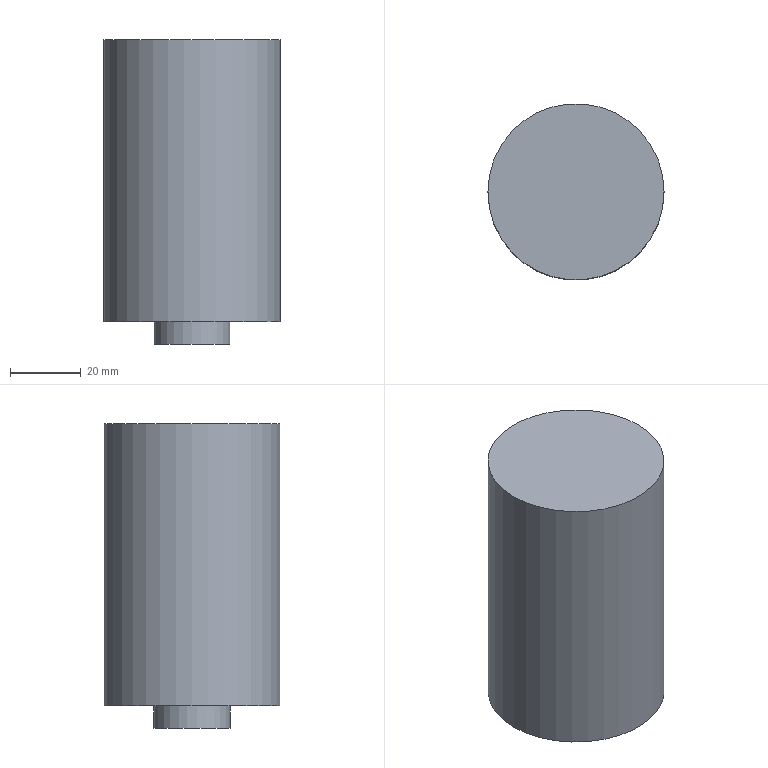Part | NX | features solid 2 | 1 solid | 5 faces | box 49.947 x 49.947 x 86.345 mm | volume 159066 mm3 | plane 3 | cylinder 2 | commonest cylinder face diameters 21.573 x1 49.947 x1
STEP:
#1=CARTESIAN_POINT('',(-1470.026,-350.026,-125.));
#2=VERTEX_POINT('',#1);
#3=CARTESIAN_POINT('',(-1495.,-350.026,-125.));
#4=DIRECTION('',(0.,0.,1.));
#5=DIRECTION('',(1.,0.,0.));
#6=AXIS2_PLACEMENT_3D('',#3,#4,#5);
#7=CIRCLE('',#6,24.974);
#8=EDGE_CURVE('',#2,#2,#7,.F.);
#9=ORIENTED_EDGE('',*,*,#8,.T.);
#10=EDGE_LOOP('',(#9));
#11=FACE_BOUND('',#10,.T.);
#12=CARTESIAN_POINT('',(-1470.026,-350.026,-205.));
#13=VERTEX_POINT('',#12);
#14=CARTESIAN_POINT('',(-1495.,-350.026,-205.));
#15=DIRECTION('',(0.,0.,1.));
#16=DIRECTION('',(1.,0.,0.));
#17=AXIS2_PLACEMENT_3D('',#14,#15,#16);
#18=CIRCLE('',#17,24.974);
#19=EDGE_CURVE('',#13,#13,#18,.F.);
#20=ORIENTED_EDGE('',*,*,#19,.F.);
#21=EDGE_LOOP('',(#20));
#22=FACE_BOUND('',#21,.T.);
#23=CARTESIAN_POINT('',(-1495.,-350.026,-141.55));
#24=DIRECTION('',(0.,0.,-1.));
#25=DIRECTION('',(0.,1.,0.));
#26=AXIS2_PLACEMENT_3D('',#23,#24,#25);
#27=CYLINDRICAL_SURFACE('',#26,24.974);
#28=ADVANCED_FACE('',(#11,#22),#27,.T.);
#29=CARTESIAN_POINT('',(-1495.,-360.813,-205.));
#30=VERTEX_POINT('',#29);
#31=CARTESIAN_POINT('',(-1495.,-350.026,-205.));
#32=DIRECTION('',(0.,0.,-1.));
#33=DIRECTION('',(0.,-1.,0.));
#34=AXIS2_PLACEMENT_3D('',#31,#32,#33);
#35=CIRCLE('',#34,10.787);
#36=EDGE_CURVE('',#30,#30,#35,.T.);
#37=ORIENTED_EDGE('',*,*,#36,.F.);
#38=EDGE_LOOP('',(#37));
#39=FACE_BOUND('',#38,.T.);
#40=ORIENTED_EDGE('',*,*,#19,.T.);
#41=EDGE_LOOP('',(#40));
#42=FACE_BOUND('',#41,.T.);
#43=CARTESIAN_POINT('',(-1495.,-350.026,-205.));
#44=DIRECTION('',(0.,0.,1.));
#45=DIRECTION('',(0.,-1.,0.));
#46=AXIS2_PLACEMENT_3D('',#43,#44,#45);
#47=PLANE('',#46);
#48=ADVANCED_FACE('',(#39,#42),#47,.F.);
#49=CARTESIAN_POINT('',(-1495.,-360.813,-211.345));
#50=VERTEX_POINT('',#49);
#51=CARTESIAN_POINT('',(-1495.,-350.026,-211.345));
#52=DIRECTION('',(0.,0.,-1.));
#53=DIRECTION('',(0.,-1.,0.));
#54=AXIS2_PLACEMENT_3D('',#51,#52,#53);
#55=CIRCLE('',#54,10.787);
#56=EDGE_CURVE('',#50,#50,#55,.T.);
#57=ORIENTED_EDGE('',*,*,#56,.F.);
#58=EDGE_LOOP('',(#57));
#59=FACE_BOUND('',#58,.T.);
#60=ORIENTED_EDGE('',*,*,#36,.T.);
#61=EDGE_LOOP('',(#60));
#62=FACE_BOUND('',#61,.T.);
#63=CARTESIAN_POINT('',(-1495.,-350.026,-211.345));
#64=DIRECTION('',(0.,0.,1.));
#65=DIRECTION('',(0.,-1.,0.));
#66=AXIS2_PLACEMENT_3D('',#63,#64,#65);
#67=CYLINDRICAL_SURFACE('',#66,10.787);
#68=ADVANCED_FACE('',(#59,#62),#67,.T.);
#69=ORIENTED_EDGE('',*,*,#56,.T.);
#70=EDGE_LOOP('',(#69));
#71=FACE_BOUND('',#70,.T.);
#72=CARTESIAN_POINT('',(-1495.,-350.026,-211.345));
#73=DIRECTION('',(0.,0.,1.));
#74=DIRECTION('',(0.,-1.,0.));
#75=AXIS2_PLACEMENT_3D('',#72,#73,#74);
#76=PLANE('',#75);
#77=ADVANCED_FACE('',(#71),#76,.F.);
#78=ORIENTED_EDGE('',*,*,#8,.F.);
#79=EDGE_LOOP('',(#78));
#80=FACE_BOUND('',#79,.T.);
#81=CARTESIAN_POINT('',(-1495.,-350.026,-125.));
#82=DIRECTION('',(0.,0.,1.));
#83=DIRECTION('',(0.,-1.,0.));
#84=AXIS2_PLACEMENT_3D('',#81,#82,#83);
#85=PLANE('',#84);
#86=ADVANCED_FACE('',(#80),#85,.T.);
#87=CLOSED_SHELL('',(#28,#48,#68,#77,#86));
#88=MANIFOLD_SOLID_BREP('',#87);
#89=(LENGTH_UNIT()NAMED_UNIT(*)SI_UNIT(.MILLI.,.METRE.));
#90=UNCERTAINTY_MEASURE_WITH_UNIT(LENGTH_MEASURE(0.00001),#89,'','');
#91=(NAMED_UNIT(*)PLANE_ANGLE_UNIT()SI_UNIT($,.RADIAN.));
#92=(NAMED_UNIT(*)SI_UNIT($,.STERADIAN.)SOLID_ANGLE_UNIT());
#93=(GEOMETRIC_REPRESENTATION_CONTEXT(3)GLOBAL_UNCERTAINTY_ASSIGNED_CONTEXT((#90))GLOBAL_UNIT_ASSIGNED_CONTEXT((#89,#91,#92))REPRESENTATION_CONTEXT('',''));
#94=ADVANCED_BREP_SHAPE_REPRESENTATION('',(#88),#93);